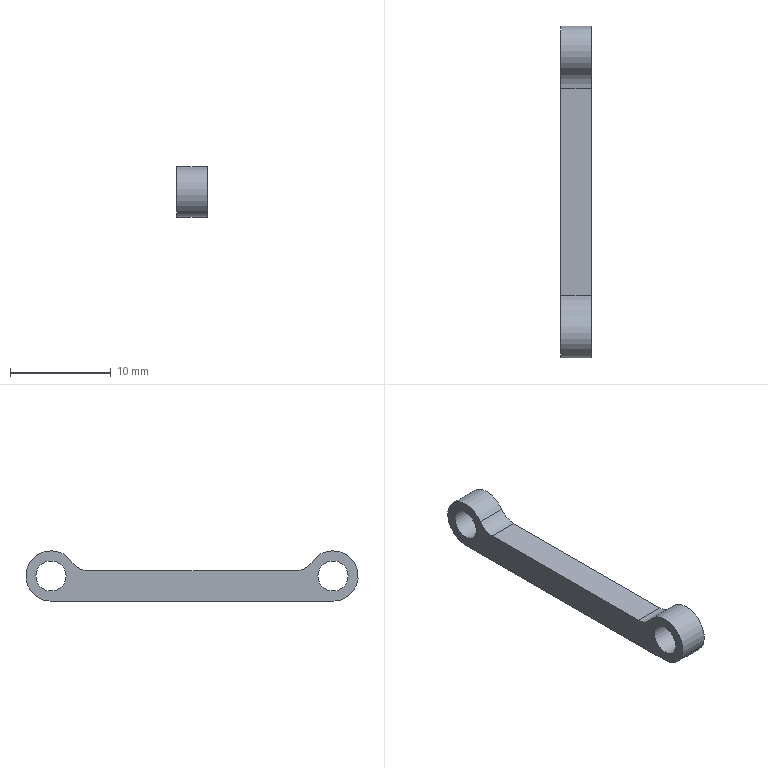Part | STEP file | 1-40.7 | 1 solid | 10 faces | box 3 x 33 x 5 mm | volume 291.958 mm3 | cylinder 6 | plane 4 | commonest cylinder face diameters 3 x2 4 x2 5 x2
STEP:
#1=CARTESIAN_POINT('',(0.,0.,0.));
#2=DIRECTION('',(0.,0.,1.));
#3=DIRECTION('',(1.,0.,0.));
#4=AXIS2_PLACEMENT_3D('',#1,#2,#3);
#5=CARTESIAN_POINT('',(0.,-14.,-2.5));
#6=VERTEX_POINT('',#5);
#7=CARTESIAN_POINT('',(0.,14.,-2.5));
#8=VERTEX_POINT('',#7);
#9=CARTESIAN_POINT('',(0.,-14.,-2.5));
#10=DIRECTION('',(0.,1.,0.));
#11=VECTOR('',#10,1.);
#12=LINE('',#9,#11);
#13=CARTESIAN_POINT('',(1.5,0.,-2.5));
#14=DIRECTION('',(0.,0.,-1.));
#15=DIRECTION('',(0.,1.,0.));
#16=AXIS2_PLACEMENT_3D('',#13,#14,#15);
#17=PLANE('',#16);
#18=CARTESIAN_POINT('',(-14.,-1.5));
#19=DIRECTION('',(1.,0.));
#20=VECTOR('',#19,1.);
#21=LINE('',#18,#20);
#22=(GEOMETRIC_REPRESENTATION_CONTEXT(2)PARAMETRIC_REPRESENTATION_CONTEXT()REPRESENTATION_CONTEXT('',''));
#23=DEFINITIONAL_REPRESENTATION('',(#21),#22);
#24=PCURVE('',#17,#23);
#25=CARTESIAN_POINT('',(0.,0.,14.151));
#26=DIRECTION('',(1.,0.,0.));
#27=DIRECTION('',(0.,1.,0.));
#28=AXIS2_PLACEMENT_3D('',#25,#26,#27);
#29=PLANE('',#28);
#30=CARTESIAN_POINT('',(-14.,-16.651));
#31=DIRECTION('',(1.,0.));
#32=VECTOR('',#31,1.);
#33=LINE('',#30,#32);
#34=(GEOMETRIC_REPRESENTATION_CONTEXT(2)PARAMETRIC_REPRESENTATION_CONTEXT()REPRESENTATION_CONTEXT('',''));
#35=DEFINITIONAL_REPRESENTATION('',(#33),#34);
#36=PCURVE('',#29,#35);
#37=SURFACE_CURVE('',#12,(#24,#36),.PCURVE_S1.);
#38=EDGE_CURVE('',#6,#8,#37,.T.);
#39=ORIENTED_EDGE('',*,*,#38,.T.);
#40=CARTESIAN_POINT('',(3.,14.,-2.5));
#41=VERTEX_POINT('',#40);
#42=CARTESIAN_POINT('',(0.,14.,-2.5));
#43=DIRECTION('',(1.,0.,0.));
#44=VECTOR('',#43,1.);
#45=LINE('',#42,#44);
#46=CARTESIAN_POINT('',(14.,-1.5));
#47=DIRECTION('',(0.,1.));
#48=VECTOR('',#47,1.);
#49=LINE('',#46,#48);
#50=(GEOMETRIC_REPRESENTATION_CONTEXT(2)PARAMETRIC_REPRESENTATION_CONTEXT()REPRESENTATION_CONTEXT('',''));
#51=DEFINITIONAL_REPRESENTATION('',(#49),#50);
#52=PCURVE('',#17,#51);
#53=CARTESIAN_POINT('',(0.,14.,0.));
#54=DIRECTION('',(1.,0.,0.));
#55=DIRECTION('',(0.,0.,-1.));
#56=AXIS2_PLACEMENT_3D('',#53,#54,#55);
#57=CYLINDRICAL_SURFACE('',#56,2.5);
#58=CARTESIAN_POINT('',(0.,0.));
#59=DIRECTION('',(0.,1.));
#60=VECTOR('',#59,1.);
#61=LINE('',#58,#60);
#62=(GEOMETRIC_REPRESENTATION_CONTEXT(2)PARAMETRIC_REPRESENTATION_CONTEXT()REPRESENTATION_CONTEXT('',''));
#63=DEFINITIONAL_REPRESENTATION('',(#61),#62);
#64=PCURVE('',#57,#63);
#65=SURFACE_CURVE('',#45,(#52,#64),.PCURVE_S1.);
#66=EDGE_CURVE('',#8,#41,#65,.T.);
#67=ORIENTED_EDGE('',*,*,#66,.T.);
#68=CARTESIAN_POINT('',(3.,-14.,-2.5));
#69=VERTEX_POINT('',#68);
#70=CARTESIAN_POINT('',(3.,-14.,-2.5));
#71=DIRECTION('',(0.,1.,0.));
#72=VECTOR('',#71,1.);
#73=LINE('',#70,#72);
#74=CARTESIAN_POINT('',(-14.,1.5));
#75=DIRECTION('',(1.,0.));
#76=VECTOR('',#75,1.);
#77=LINE('',#74,#76);
#78=(GEOMETRIC_REPRESENTATION_CONTEXT(2)PARAMETRIC_REPRESENTATION_CONTEXT()REPRESENTATION_CONTEXT('',''));
#79=DEFINITIONAL_REPRESENTATION('',(#77),#78);
#80=PCURVE('',#17,#79);
#81=CARTESIAN_POINT('',(3.,0.,14.151));
#82=DIRECTION('',(1.,0.,0.));
#83=DIRECTION('',(0.,1.,0.));
#84=AXIS2_PLACEMENT_3D('',#81,#82,#83);
#85=PLANE('',#84);
#86=CARTESIAN_POINT('',(-14.,-16.651));
#87=DIRECTION('',(1.,0.));
#88=VECTOR('',#87,1.);
#89=LINE('',#86,#88);
#90=(GEOMETRIC_REPRESENTATION_CONTEXT(2)PARAMETRIC_REPRESENTATION_CONTEXT()REPRESENTATION_CONTEXT('',''));
#91=DEFINITIONAL_REPRESENTATION('',(#89),#90);
#92=PCURVE('',#85,#91);
#93=SURFACE_CURVE('',#73,(#80,#92),.PCURVE_S1.);
#94=EDGE_CURVE('',#69,#41,#93,.T.);
#95=ORIENTED_EDGE('',*,*,#94,.F.);
#96=CARTESIAN_POINT('',(0.,-14.,-2.5));
#97=DIRECTION('',(1.,0.,0.));
#98=VECTOR('',#97,1.);
#99=LINE('',#96,#98);
#100=CARTESIAN_POINT('',(-14.,-1.5));
#101=DIRECTION('',(0.,1.));
#102=VECTOR('',#101,1.);
#103=LINE('',#100,#102);
#104=(GEOMETRIC_REPRESENTATION_CONTEXT(2)PARAMETRIC_REPRESENTATION_CONTEXT()REPRESENTATION_CONTEXT('',''));
#105=DEFINITIONAL_REPRESENTATION('',(#103),#104);
#106=PCURVE('',#17,#105);
#107=CARTESIAN_POINT('',(0.,-14.,0.));
#108=DIRECTION('',(1.,0.,0.));
#109=DIRECTION('',(0.,0.9798,0.2));
#110=AXIS2_PLACEMENT_3D('',#107,#108,#109);
#111=CYLINDRICAL_SURFACE('',#110,2.5);
#112=CARTESIAN_POINT('',(4.511,0.));
#113=DIRECTION('',(0.,1.));
#114=VECTOR('',#113,1.);
#115=LINE('',#112,#114);
#116=(GEOMETRIC_REPRESENTATION_CONTEXT(2)PARAMETRIC_REPRESENTATION_CONTEXT()REPRESENTATION_CONTEXT('',''));
#117=DEFINITIONAL_REPRESENTATION('',(#115),#116);
#118=PCURVE('',#111,#117);
#119=SURFACE_CURVE('',#99,(#106,#118),.PCURVE_S1.);
#120=EDGE_CURVE('',#6,#69,#119,.T.);
#121=ORIENTED_EDGE('',*,*,#120,.F.);
#122=EDGE_LOOP('',(#39,#67,#95,#121));
#123=FACE_BOUND('',#122,.T.);
#124=ADVANCED_FACE('',(#123),#17,.T.);
#125=CARTESIAN_POINT('',(0.,-12.5,0.));
#126=VERTEX_POINT('',#125);
#127=CARTESIAN_POINT('',(3.,-12.5,0.));
#128=VERTEX_POINT('',#127);
#129=CARTESIAN_POINT('',(0.,-12.5,0.));
#130=DIRECTION('',(1.,0.,0.));
#131=VECTOR('',#130,1.);
#132=LINE('',#129,#131);
#133=CARTESIAN_POINT('',(0.,-14.,0.));
#134=DIRECTION('',(1.,0.,0.));
#135=DIRECTION('',(0.,1.,0.));
#136=AXIS2_PLACEMENT_3D('',#133,#134,#135);
#137=CYLINDRICAL_SURFACE('',#136,1.5);
#138=CARTESIAN_POINT('',(6.283,0.));
#139=DIRECTION('',(0.,1.));
#140=VECTOR('',#139,1.);
#141=LINE('',#138,#140);
#142=(GEOMETRIC_REPRESENTATION_CONTEXT(2)PARAMETRIC_REPRESENTATION_CONTEXT()REPRESENTATION_CONTEXT('',''));
#143=DEFINITIONAL_REPRESENTATION('',(#141),#142);
#144=PCURVE('',#137,#143);
#145=CARTESIAN_POINT('',(0.,0.));
#146=DIRECTION('',(0.,1.));
#147=VECTOR('',#146,1.);
#148=LINE('',#145,#147);
#149=(GEOMETRIC_REPRESENTATION_CONTEXT(2)PARAMETRIC_REPRESENTATION_CONTEXT()REPRESENTATION_CONTEXT('',''));
#150=DEFINITIONAL_REPRESENTATION('',(#148),#149);
#151=PCURVE('',#137,#150);
#152=SEAM_CURVE('',#132,(#144,#151),.PCURVE_S1.);
#153=EDGE_CURVE('',#126,#128,#152,.T.);
#154=ORIENTED_EDGE('',*,*,#153,.T.);
#155=CARTESIAN_POINT('',(3.,-14.,0.));
#156=DIRECTION('',(-1.,0.,0.));
#157=DIRECTION('',(0.,1.,0.));
#158=AXIS2_PLACEMENT_3D('',#155,#156,#157);
#159=CIRCLE('',#158,1.5);
#160=CARTESIAN_POINT('',(6.283,3.));
#161=DIRECTION('',(-1.,0.));
#162=VECTOR('',#161,1.);
#163=LINE('',#160,#162);
#164=(GEOMETRIC_REPRESENTATION_CONTEXT(2)PARAMETRIC_REPRESENTATION_CONTEXT()REPRESENTATION_CONTEXT('',''));
#165=DEFINITIONAL_REPRESENTATION('',(#163),#164);
#166=PCURVE('',#137,#165);
#167=CARTESIAN_POINT('',(-12.5,-14.151));
#168=CARTESIAN_POINT('',(-12.5,-16.749));
#169=CARTESIAN_POINT('',(-14.75,-15.45));
#170=CARTESIAN_POINT('',(-17.,-14.151));
#171=CARTESIAN_POINT('',(-14.75,-12.852));
#172=CARTESIAN_POINT('',(-12.5,-11.553));
#173=CARTESIAN_POINT('',(-12.5,-14.151));
#174=(BOUNDED_CURVE()B_SPLINE_CURVE(2,(#167,#168,#169,#170,#171,#172,#173),.UNSPECIFIED.,.T.,.F.)B_SPLINE_CURVE_WITH_KNOTS((1,2,2,2,2,1),(-2.094,0.,2.094,4.189,6.283,8.378),.UNSPECIFIED.)CURVE()GEOMETRIC_REPRESENTATION_ITEM()RATIONAL_B_SPLINE_CURVE((1.,0.5,1.,0.5,1.,0.5,1.))REPRESENTATION_ITEM(''));
#175=(GEOMETRIC_REPRESENTATION_CONTEXT(2)PARAMETRIC_REPRESENTATION_CONTEXT()REPRESENTATION_CONTEXT('',''));
#176=DEFINITIONAL_REPRESENTATION('',(#174),#175);
#177=PCURVE('',#85,#176);
#178=SURFACE_CURVE('',#159,(#166,#177),.PCURVE_S1.);
#179=EDGE_CURVE('',#128,#128,#178,.T.);
#180=ORIENTED_EDGE('',*,*,#179,.T.);
#181=ORIENTED_EDGE('',*,*,#153,.F.);
#182=CARTESIAN_POINT('',(0.,-14.,0.));
#183=DIRECTION('',(-1.,0.,0.));
#184=DIRECTION('',(0.,1.,0.));
#185=AXIS2_PLACEMENT_3D('',#182,#183,#184);
#186=CIRCLE('',#185,1.5);
#187=CARTESIAN_POINT('',(6.283,0.));
#188=DIRECTION('',(-1.,0.));
#189=VECTOR('',#188,1.);
#190=LINE('',#187,#189);
#191=(GEOMETRIC_REPRESENTATION_CONTEXT(2)PARAMETRIC_REPRESENTATION_CONTEXT()REPRESENTATION_CONTEXT('',''));
#192=DEFINITIONAL_REPRESENTATION('',(#190),#191);
#193=PCURVE('',#137,#192);
#194=CARTESIAN_POINT('',(-12.5,-14.151));
#195=CARTESIAN_POINT('',(-12.5,-16.749));
#196=CARTESIAN_POINT('',(-14.75,-15.45));
#197=CARTESIAN_POINT('',(-17.,-14.151));
#198=CARTESIAN_POINT('',(-14.75,-12.852));
#199=CARTESIAN_POINT('',(-12.5,-11.553));
#200=CARTESIAN_POINT('',(-12.5,-14.151));
#201=(BOUNDED_CURVE()B_SPLINE_CURVE(2,(#194,#195,#196,#197,#198,#199,#200),.UNSPECIFIED.,.T.,.F.)B_SPLINE_CURVE_WITH_KNOTS((1,2,2,2,2,1),(-2.094,0.,2.094,4.189,6.283,8.378),.UNSPECIFIED.)CURVE()GEOMETRIC_REPRESENTATION_ITEM()RATIONAL_B_SPLINE_CURVE((1.,0.5,1.,0.5,1.,0.5,1.))REPRESENTATION_ITEM(''));
#202=(GEOMETRIC_REPRESENTATION_CONTEXT(2)PARAMETRIC_REPRESENTATION_CONTEXT()REPRESENTATION_CONTEXT('',''));
#203=DEFINITIONAL_REPRESENTATION('',(#201),#202);
#204=PCURVE('',#29,#203);
#205=SURFACE_CURVE('',#186,(#193,#204),.PCURVE_S1.);
#206=EDGE_CURVE('',#126,#126,#205,.T.);
#207=ORIENTED_EDGE('',*,*,#206,.F.);
#208=EDGE_LOOP('',(#154,#180,#181,#207));
#209=FACE_BOUND('',#208,.F.);
#210=ADVANCED_FACE('',(#209),#137,.F.);
#211=CARTESIAN_POINT('',(0.,15.5,0.));
#212=VERTEX_POINT('',#211);
#213=CARTESIAN_POINT('',(3.,15.5,0.));
#214=VERTEX_POINT('',#213);
#215=CARTESIAN_POINT('',(0.,15.5,0.));
#216=DIRECTION('',(1.,0.,0.));
#217=VECTOR('',#216,1.);
#218=LINE('',#215,#217);
#219=CARTESIAN_POINT('',(0.,14.,0.));
#220=DIRECTION('',(1.,0.,0.));
#221=DIRECTION('',(0.,1.,0.));
#222=AXIS2_PLACEMENT_3D('',#219,#220,#221);
#223=CYLINDRICAL_SURFACE('',#222,1.5);
#224=CARTESIAN_POINT('',(6.283,0.));
#225=DIRECTION('',(0.,1.));
#226=VECTOR('',#225,1.);
#227=LINE('',#224,#226);
#228=(GEOMETRIC_REPRESENTATION_CONTEXT(2)PARAMETRIC_REPRESENTATION_CONTEXT()REPRESENTATION_CONTEXT('',''));
#229=DEFINITIONAL_REPRESENTATION('',(#227),#228);
#230=PCURVE('',#223,#229);
#231=CARTESIAN_POINT('',(0.,0.));
#232=DIRECTION('',(0.,1.));
#233=VECTOR('',#232,1.);
#234=LINE('',#231,#233);
#235=(GEOMETRIC_REPRESENTATION_CONTEXT(2)PARAMETRIC_REPRESENTATION_CONTEXT()REPRESENTATION_CONTEXT('',''));
#236=DEFINITIONAL_REPRESENTATION('',(#234),#235);
#237=PCURVE('',#223,#236);
#238=SEAM_CURVE('',#218,(#230,#237),.PCURVE_S1.);
#239=EDGE_CURVE('',#212,#214,#238,.T.);
#240=ORIENTED_EDGE('',*,*,#239,.T.);
#241=CARTESIAN_POINT('',(3.,14.,0.));
#242=DIRECTION('',(-1.,0.,0.));
#243=DIRECTION('',(0.,1.,0.));
#244=AXIS2_PLACEMENT_3D('',#241,#242,#243);
#245=CIRCLE('',#244,1.5);
#246=CARTESIAN_POINT('',(6.283,3.));
#247=DIRECTION('',(-1.,0.));
#248=VECTOR('',#247,1.);
#249=LINE('',#246,#248);
#250=(GEOMETRIC_REPRESENTATION_CONTEXT(2)PARAMETRIC_REPRESENTATION_CONTEXT()REPRESENTATION_CONTEXT('',''));
#251=DEFINITIONAL_REPRESENTATION('',(#249),#250);
#252=PCURVE('',#223,#251);
#253=CARTESIAN_POINT('',(15.5,-14.151));
#254=CARTESIAN_POINT('',(15.5,-16.749));
#255=CARTESIAN_POINT('',(13.25,-15.45));
#256=CARTESIAN_POINT('',(11.,-14.151));
#257=CARTESIAN_POINT('',(13.25,-12.852));
#258=CARTESIAN_POINT('',(15.5,-11.553));
#259=CARTESIAN_POINT('',(15.5,-14.151));
#260=(BOUNDED_CURVE()B_SPLINE_CURVE(2,(#253,#254,#255,#256,#257,#258,#259),.UNSPECIFIED.,.T.,.F.)B_SPLINE_CURVE_WITH_KNOTS((1,2,2,2,2,1),(-2.094,0.,2.094,4.189,6.283,8.378),.UNSPECIFIED.)CURVE()GEOMETRIC_REPRESENTATION_ITEM()RATIONAL_B_SPLINE_CURVE((1.,0.5,1.,0.5,1.,0.5,1.))REPRESENTATION_ITEM(''));
#261=(GEOMETRIC_REPRESENTATION_CONTEXT(2)PARAMETRIC_REPRESENTATION_CONTEXT()REPRESENTATION_CONTEXT('',''));
#262=DEFINITIONAL_REPRESENTATION('',(#260),#261);
#263=PCURVE('',#85,#262);
#264=SURFACE_CURVE('',#245,(#252,#263),.PCURVE_S1.);
#265=EDGE_CURVE('',#214,#214,#264,.T.);
#266=ORIENTED_EDGE('',*,*,#265,.T.);
#267=ORIENTED_EDGE('',*,*,#239,.F.);
#268=CARTESIAN_POINT('',(0.,14.,0.));
#269=DIRECTION('',(-1.,0.,0.));
#270=DIRECTION('',(0.,1.,0.));
#271=AXIS2_PLACEMENT_3D('',#268,#269,#270);
#272=CIRCLE('',#271,1.5);
#273=CARTESIAN_POINT('',(6.283,0.));
#274=DIRECTION('',(-1.,0.));
#275=VECTOR('',#274,1.);
#276=LINE('',#273,#275);
#277=(GEOMETRIC_REPRESENTATION_CONTEXT(2)PARAMETRIC_REPRESENTATION_CONTEXT()REPRESENTATION_CONTEXT('',''));
#278=DEFINITIONAL_REPRESENTATION('',(#276),#277);
#279=PCURVE('',#223,#278);
#280=CARTESIAN_POINT('',(15.5,-14.151));
#281=CARTESIAN_POINT('',(15.5,-16.749));
#282=CARTESIAN_POINT('',(13.25,-15.45));
#283=CARTESIAN_POINT('',(11.,-14.151));
#284=CARTESIAN_POINT('',(13.25,-12.852));
#285=CARTESIAN_POINT('',(15.5,-11.553));
#286=CARTESIAN_POINT('',(15.5,-14.151));
#287=(BOUNDED_CURVE()B_SPLINE_CURVE(2,(#280,#281,#282,#283,#284,#285,#286),.UNSPECIFIED.,.T.,.F.)B_SPLINE_CURVE_WITH_KNOTS((1,2,2,2,2,1),(-2.094,0.,2.094,4.189,6.283,8.378),.UNSPECIFIED.)CURVE()GEOMETRIC_REPRESENTATION_ITEM()RATIONAL_B_SPLINE_CURVE((1.,0.5,1.,0.5,1.,0.5,1.))REPRESENTATION_ITEM(''));
#288=(GEOMETRIC_REPRESENTATION_CONTEXT(2)PARAMETRIC_REPRESENTATION_CONTEXT()REPRESENTATION_CONTEXT('',''));
#289=DEFINITIONAL_REPRESENTATION('',(#287),#288);
#290=PCURVE('',#29,#289);
#291=SURFACE_CURVE('',#272,(#279,#290),.PCURVE_S1.);
#292=EDGE_CURVE('',#212,#212,#291,.T.);
#293=ORIENTED_EDGE('',*,*,#292,.F.);
#294=EDGE_LOOP('',(#240,#266,#267,#293));
#295=FACE_BOUND('',#294,.F.);
#296=ADVANCED_FACE('',(#295),#223,.F.);
#297=CARTESIAN_POINT('',(0.,10.258,0.5));
#298=VERTEX_POINT('',#297);
#299=CARTESIAN_POINT('',(0.,-10.258,0.5));
#300=VERTEX_POINT('',#299);
#301=CARTESIAN_POINT('',(0.,10.258,0.5));
#302=DIRECTION('',(0.,-1.,0.));
#303=VECTOR('',#302,1.);
#304=LINE('',#301,#303);
#305=CARTESIAN_POINT('',(10.258,-13.651));
#306=DIRECTION('',(-1.,0.));
#307=VECTOR('',#306,1.);
#308=LINE('',#305,#307);
#309=(GEOMETRIC_REPRESENTATION_CONTEXT(2)PARAMETRIC_REPRESENTATION_CONTEXT()REPRESENTATION_CONTEXT('',''));
#310=DEFINITIONAL_REPRESENTATION('',(#308),#309);
#311=PCURVE('',#29,#310);
#312=CARTESIAN_POINT('',(1.5,0.,0.5));
#313=DIRECTION('',(0.,0.,1.));
#314=DIRECTION('',(0.,-1.,0.));
#315=AXIS2_PLACEMENT_3D('',#312,#313,#314);
#316=PLANE('',#315);
#317=CARTESIAN_POINT('',(-10.258,-1.5));
#318=DIRECTION('',(1.,0.));
#319=VECTOR('',#318,1.);
#320=LINE('',#317,#319);
#321=(GEOMETRIC_REPRESENTATION_CONTEXT(2)PARAMETRIC_REPRESENTATION_CONTEXT()REPRESENTATION_CONTEXT('',''));
#322=DEFINITIONAL_REPRESENTATION('',(#320),#321);
#323=PCURVE('',#316,#322);
#324=SURFACE_CURVE('',#304,(#311,#323),.PCURVE_S1.);
#325=EDGE_CURVE('',#298,#300,#324,.T.);
#326=ORIENTED_EDGE('',*,*,#325,.T.);
#327=CARTESIAN_POINT('',(0.,-11.921,1.389));
#328=VERTEX_POINT('',#327);
#329=CARTESIAN_POINT('',(0.,-10.258,2.5));
#330=DIRECTION('',(-1.,0.,0.));
#331=DIRECTION('',(0.,0.,-1.));
#332=AXIS2_PLACEMENT_3D('',#329,#330,#331);
#333=CIRCLE('',#332,2.);
#334=CARTESIAN_POINT('',(-10.258,-13.651));
#335=CARTESIAN_POINT('',(-13.722,-13.651));
#336=CARTESIAN_POINT('',(-11.99,-10.651));
#337=CARTESIAN_POINT('',(-10.258,-7.651));
#338=CARTESIAN_POINT('',(-8.526,-10.651));
#339=CARTESIAN_POINT('',(-6.794,-13.651));
#340=CARTESIAN_POINT('',(-10.258,-13.651));
#341=(BOUNDED_CURVE()B_SPLINE_CURVE(2,(#334,#335,#336,#337,#338,#339,#340),.UNSPECIFIED.,.T.,.F.)B_SPLINE_CURVE_WITH_KNOTS((1,2,2,2,2,1),(-2.094,0.,2.094,4.189,6.283,8.378),.UNSPECIFIED.)CURVE()GEOMETRIC_REPRESENTATION_ITEM()RATIONAL_B_SPLINE_CURVE((1.,0.5,1.,0.5,1.,0.5,1.))REPRESENTATION_ITEM(''));
#342=(GEOMETRIC_REPRESENTATION_CONTEXT(2)PARAMETRIC_REPRESENTATION_CONTEXT()REPRESENTATION_CONTEXT('',''));
#343=DEFINITIONAL_REPRESENTATION('',(#341),#342);
#344=PCURVE('',#29,#343);
#345=CARTESIAN_POINT('',(0.,-10.258,2.5));
#346=DIRECTION('',(1.,0.,0.));
#347=DIRECTION('',(0.,0.,-1.));
#348=AXIS2_PLACEMENT_3D('',#345,#346,#347);
#349=CYLINDRICAL_SURFACE('',#348,2.);
#350=CARTESIAN_POINT('',(6.283,0.));
#351=DIRECTION('',(-1.,0.));
#352=VECTOR('',#351,1.);
#353=LINE('',#350,#352);
#354=(GEOMETRIC_REPRESENTATION_CONTEXT(2)PARAMETRIC_REPRESENTATION_CONTEXT()REPRESENTATION_CONTEXT('',''));
#355=DEFINITIONAL_REPRESENTATION('',(#353),#354);
#356=PCURVE('',#349,#355);
#357=SURFACE_CURVE('',#333,(#344,#356),.PCURVE_S1.);
#358=EDGE_CURVE('',#300,#328,#357,.T.);
#359=ORIENTED_EDGE('',*,*,#358,.T.);
#360=CARTESIAN_POINT('',(0.,-14.,0.));
#361=DIRECTION('',(1.,0.,0.));
#362=DIRECTION('',(0.,0.8315,0.5556));
#363=AXIS2_PLACEMENT_3D('',#360,#361,#362);
#364=CIRCLE('',#363,2.5);
#365=CARTESIAN_POINT('',(-14.,-14.151));
#366=DIRECTION('',(0.8315,0.5556));
#367=AXIS2_PLACEMENT_2D('',#365,#366);
#368=CIRCLE('',#367,2.5);
#369=(GEOMETRIC_REPRESENTATION_CONTEXT(2)PARAMETRIC_REPRESENTATION_CONTEXT()REPRESENTATION_CONTEXT('',''));
#370=DEFINITIONAL_REPRESENTATION('',(#368),#369);
#371=PCURVE('',#29,#370);
#372=CARTESIAN_POINT('',(0.3877,0.));
#373=DIRECTION('',(1.,0.));
#374=VECTOR('',#373,1.);
#375=LINE('',#372,#374);
#376=(GEOMETRIC_REPRESENTATION_CONTEXT(2)PARAMETRIC_REPRESENTATION_CONTEXT()REPRESENTATION_CONTEXT('',''));
#377=DEFINITIONAL_REPRESENTATION('',(#375),#376);
#378=PCURVE('',#111,#377);
#379=SURFACE_CURVE('',#364,(#371,#378),.PCURVE_S1.);
#380=EDGE_CURVE('',#328,#6,#379,.T.);
#381=ORIENTED_EDGE('',*,*,#380,.T.);
#382=ORIENTED_EDGE('',*,*,#38,.T.);
#383=CARTESIAN_POINT('',(0.,11.921,1.389));
#384=VERTEX_POINT('',#383);
#385=CARTESIAN_POINT('',(0.,14.,0.));
#386=DIRECTION('',(1.,0.,0.));
#387=DIRECTION('',(0.,0.,-1.));
#388=AXIS2_PLACEMENT_3D('',#385,#386,#387);
#389=CIRCLE('',#388,2.5);
#390=CARTESIAN_POINT('',(14.,-14.151));
#391=DIRECTION('',(0.,-1.));
#392=AXIS2_PLACEMENT_2D('',#390,#391);
#393=CIRCLE('',#392,2.5);
#394=(GEOMETRIC_REPRESENTATION_CONTEXT(2)PARAMETRIC_REPRESENTATION_CONTEXT()REPRESENTATION_CONTEXT('',''));
#395=DEFINITIONAL_REPRESENTATION('',(#393),#394);
#396=PCURVE('',#29,#395);
#397=CARTESIAN_POINT('',(0.,0.));
#398=DIRECTION('',(1.,0.));
#399=VECTOR('',#398,1.);
#400=LINE('',#397,#399);
#401=(GEOMETRIC_REPRESENTATION_CONTEXT(2)PARAMETRIC_REPRESENTATION_CONTEXT()REPRESENTATION_CONTEXT('',''));
#402=DEFINITIONAL_REPRESENTATION('',(#400),#401);
#403=PCURVE('',#57,#402);
#404=SURFACE_CURVE('',#389,(#396,#403),.PCURVE_S1.);
#405=EDGE_CURVE('',#8,#384,#404,.T.);
#406=ORIENTED_EDGE('',*,*,#405,.T.);
#407=CARTESIAN_POINT('',(0.,10.258,2.5));
#408=DIRECTION('',(-1.,0.,0.));
#409=DIRECTION('',(0.,0.8315,-0.5556));
#410=AXIS2_PLACEMENT_3D('',#407,#408,#409);
#411=CIRCLE('',#410,2.);
#412=CARTESIAN_POINT('',(11.921,-12.762));
#413=CARTESIAN_POINT('',(9.997,-15.643));
#414=CARTESIAN_POINT('',(8.465,-12.536));
#415=CARTESIAN_POINT('',(6.932,-9.429));
#416=CARTESIAN_POINT('',(10.389,-9.655));
#417=CARTESIAN_POINT('',(13.846,-9.882));
#418=CARTESIAN_POINT('',(11.921,-12.762));
#419=(BOUNDED_CURVE()B_SPLINE_CURVE(2,(#412,#413,#414,#415,#416,#417,#418),.UNSPECIFIED.,.T.,.F.)B_SPLINE_CURVE_WITH_KNOTS((1,2,2,2,2,1),(-2.094,0.,2.094,4.189,6.283,8.378),.UNSPECIFIED.)CURVE()GEOMETRIC_REPRESENTATION_ITEM()RATIONAL_B_SPLINE_CURVE((1.,0.5,1.,0.5,1.,0.5,1.))REPRESENTATION_ITEM(''));
#420=(GEOMETRIC_REPRESENTATION_CONTEXT(2)PARAMETRIC_REPRESENTATION_CONTEXT()REPRESENTATION_CONTEXT('',''));
#421=DEFINITIONAL_REPRESENTATION('',(#419),#420);
#422=PCURVE('',#29,#421);
#423=CARTESIAN_POINT('',(0.,10.258,2.5));
#424=DIRECTION('',(1.,0.,0.));
#425=DIRECTION('',(0.,0.8315,-0.5556));
#426=AXIS2_PLACEMENT_3D('',#423,#424,#425);
#427=CYLINDRICAL_SURFACE('',#426,2.);
#428=CARTESIAN_POINT('',(6.283,0.));
#429=DIRECTION('',(-1.,0.));
#430=VECTOR('',#429,1.);
#431=LINE('',#428,#430);
#432=(GEOMETRIC_REPRESENTATION_CONTEXT(2)PARAMETRIC_REPRESENTATION_CONTEXT()REPRESENTATION_CONTEXT('',''));
#433=DEFINITIONAL_REPRESENTATION('',(#431),#432);
#434=PCURVE('',#427,#433);
#435=SURFACE_CURVE('',#411,(#422,#434),.PCURVE_S1.);
#436=EDGE_CURVE('',#384,#298,#435,.T.);
#437=ORIENTED_EDGE('',*,*,#436,.T.);
#438=EDGE_LOOP('',(#326,#359,#381,#382,#406,#437));
#439=FACE_BOUND('',#438,.F.);
#440=ORIENTED_EDGE('',*,*,#292,.T.);
#441=EDGE_LOOP('',(#440));
#442=FACE_BOUND('',#441,.F.);
#443=ORIENTED_EDGE('',*,*,#206,.T.);
#444=EDGE_LOOP('',(#443));
#445=FACE_BOUND('',#444,.F.);
#446=ADVANCED_FACE('',(#439,#442,#445),#29,.F.);
#447=CARTESIAN_POINT('',(3.,10.258,0.5));
#448=VERTEX_POINT('',#447);
#449=CARTESIAN_POINT('',(3.,-10.258,0.5));
#450=VERTEX_POINT('',#449);
#451=CARTESIAN_POINT('',(3.,10.258,0.5));
#452=DIRECTION('',(0.,-1.,0.));
#453=VECTOR('',#452,1.);
#454=LINE('',#451,#453);
#455=CARTESIAN_POINT('',(10.258,-13.651));
#456=DIRECTION('',(-1.,0.));
#457=VECTOR('',#456,1.);
#458=LINE('',#455,#457);
#459=(GEOMETRIC_REPRESENTATION_CONTEXT(2)PARAMETRIC_REPRESENTATION_CONTEXT()REPRESENTATION_CONTEXT('',''));
#460=DEFINITIONAL_REPRESENTATION('',(#458),#459);
#461=PCURVE('',#85,#460);
#462=CARTESIAN_POINT('',(-10.258,1.5));
#463=DIRECTION('',(1.,0.));
#464=VECTOR('',#463,1.);
#465=LINE('',#462,#464);
#466=(GEOMETRIC_REPRESENTATION_CONTEXT(2)PARAMETRIC_REPRESENTATION_CONTEXT()REPRESENTATION_CONTEXT('',''));
#467=DEFINITIONAL_REPRESENTATION('',(#465),#466);
#468=PCURVE('',#316,#467);
#469=SURFACE_CURVE('',#454,(#461,#468),.PCURVE_S1.);
#470=EDGE_CURVE('',#448,#450,#469,.T.);
#471=ORIENTED_EDGE('',*,*,#470,.T.);
#472=CARTESIAN_POINT('',(3.,-11.921,1.389));
#473=VERTEX_POINT('',#472);
#474=CARTESIAN_POINT('',(3.,-10.258,2.5));
#475=DIRECTION('',(-1.,0.,0.));
#476=DIRECTION('',(0.,0.,-1.));
#477=AXIS2_PLACEMENT_3D('',#474,#475,#476);
#478=CIRCLE('',#477,2.);
#479=CARTESIAN_POINT('',(-10.258,-13.651));
#480=CARTESIAN_POINT('',(-13.722,-13.651));
#481=CARTESIAN_POINT('',(-11.99,-10.651));
#482=CARTESIAN_POINT('',(-10.258,-7.651));
#483=CARTESIAN_POINT('',(-8.526,-10.651));
#484=CARTESIAN_POINT('',(-6.794,-13.651));
#485=CARTESIAN_POINT('',(-10.258,-13.651));
#486=(BOUNDED_CURVE()B_SPLINE_CURVE(2,(#479,#480,#481,#482,#483,#484,#485),.UNSPECIFIED.,.T.,.F.)B_SPLINE_CURVE_WITH_KNOTS((1,2,2,2,2,1),(-2.094,0.,2.094,4.189,6.283,8.378),.UNSPECIFIED.)CURVE()GEOMETRIC_REPRESENTATION_ITEM()RATIONAL_B_SPLINE_CURVE((1.,0.5,1.,0.5,1.,0.5,1.))REPRESENTATION_ITEM(''));
#487=(GEOMETRIC_REPRESENTATION_CONTEXT(2)PARAMETRIC_REPRESENTATION_CONTEXT()REPRESENTATION_CONTEXT('',''));
#488=DEFINITIONAL_REPRESENTATION('',(#486),#487);
#489=PCURVE('',#85,#488);
#490=CARTESIAN_POINT('',(6.283,3.));
#491=DIRECTION('',(-1.,0.));
#492=VECTOR('',#491,1.);
#493=LINE('',#490,#492);
#494=(GEOMETRIC_REPRESENTATION_CONTEXT(2)PARAMETRIC_REPRESENTATION_CONTEXT()REPRESENTATION_CONTEXT('',''));
#495=DEFINITIONAL_REPRESENTATION('',(#493),#494);
#496=PCURVE('',#349,#495);
#497=SURFACE_CURVE('',#478,(#489,#496),.PCURVE_S1.);
#498=EDGE_CURVE('',#450,#473,#497,.T.);
#499=ORIENTED_EDGE('',*,*,#498,.T.);
#500=CARTESIAN_POINT('',(3.,-14.,0.));
#501=DIRECTION('',(1.,0.,0.));
#502=DIRECTION('',(0.,0.8315,0.5556));
#503=AXIS2_PLACEMENT_3D('',#500,#501,#502);
#504=CIRCLE('',#503,2.5);
#505=CARTESIAN_POINT('',(-14.,-14.151));
#506=DIRECTION('',(0.8315,0.5556));
#507=AXIS2_PLACEMENT_2D('',#505,#506);
#508=CIRCLE('',#507,2.5);
#509=(GEOMETRIC_REPRESENTATION_CONTEXT(2)PARAMETRIC_REPRESENTATION_CONTEXT()REPRESENTATION_CONTEXT('',''));
#510=DEFINITIONAL_REPRESENTATION('',(#508),#509);
#511=PCURVE('',#85,#510);
#512=CARTESIAN_POINT('',(0.3877,3.));
#513=DIRECTION('',(1.,0.));
#514=VECTOR('',#513,1.);
#515=LINE('',#512,#514);
#516=(GEOMETRIC_REPRESENTATION_CONTEXT(2)PARAMETRIC_REPRESENTATION_CONTEXT()REPRESENTATION_CONTEXT('',''));
#517=DEFINITIONAL_REPRESENTATION('',(#515),#516);
#518=PCURVE('',#111,#517);
#519=SURFACE_CURVE('',#504,(#511,#518),.PCURVE_S1.);
#520=EDGE_CURVE('',#473,#69,#519,.T.);
#521=ORIENTED_EDGE('',*,*,#520,.T.);
#522=ORIENTED_EDGE('',*,*,#94,.T.);
#523=CARTESIAN_POINT('',(3.,11.921,1.389));
#524=VERTEX_POINT('',#523);
#525=CARTESIAN_POINT('',(3.,14.,0.));
#526=DIRECTION('',(1.,0.,0.));
#527=DIRECTION('',(0.,0.,-1.));
#528=AXIS2_PLACEMENT_3D('',#525,#526,#527);
#529=CIRCLE('',#528,2.5);
#530=CARTESIAN_POINT('',(14.,-14.151));
#531=DIRECTION('',(0.,-1.));
#532=AXIS2_PLACEMENT_2D('',#530,#531);
#533=CIRCLE('',#532,2.5);
#534=(GEOMETRIC_REPRESENTATION_CONTEXT(2)PARAMETRIC_REPRESENTATION_CONTEXT()REPRESENTATION_CONTEXT('',''));
#535=DEFINITIONAL_REPRESENTATION('',(#533),#534);
#536=PCURVE('',#85,#535);
#537=CARTESIAN_POINT('',(0.,3.));
#538=DIRECTION('',(1.,0.));
#539=VECTOR('',#538,1.);
#540=LINE('',#537,#539);
#541=(GEOMETRIC_REPRESENTATION_CONTEXT(2)PARAMETRIC_REPRESENTATION_CONTEXT()REPRESENTATION_CONTEXT('',''));
#542=DEFINITIONAL_REPRESENTATION('',(#540),#541);
#543=PCURVE('',#57,#542);
#544=SURFACE_CURVE('',#529,(#536,#543),.PCURVE_S1.);
#545=EDGE_CURVE('',#41,#524,#544,.T.);
#546=ORIENTED_EDGE('',*,*,#545,.T.);
#547=CARTESIAN_POINT('',(3.,10.258,2.5));
#548=DIRECTION('',(-1.,0.,0.));
#549=DIRECTION('',(0.,0.8315,-0.5556));
#550=AXIS2_PLACEMENT_3D('',#547,#548,#549);
#551=CIRCLE('',#550,2.);
#552=CARTESIAN_POINT('',(11.921,-12.762));
#553=CARTESIAN_POINT('',(9.997,-15.643));
#554=CARTESIAN_POINT('',(8.465,-12.536));
#555=CARTESIAN_POINT('',(6.932,-9.429));
#556=CARTESIAN_POINT('',(10.389,-9.655));
#557=CARTESIAN_POINT('',(13.846,-9.882));
#558=CARTESIAN_POINT('',(11.921,-12.762));
#559=(BOUNDED_CURVE()B_SPLINE_CURVE(2,(#552,#553,#554,#555,#556,#557,#558),.UNSPECIFIED.,.T.,.F.)B_SPLINE_CURVE_WITH_KNOTS((1,2,2,2,2,1),(-2.094,0.,2.094,4.189,6.283,8.378),.UNSPECIFIED.)CURVE()GEOMETRIC_REPRESENTATION_ITEM()RATIONAL_B_SPLINE_CURVE((1.,0.5,1.,0.5,1.,0.5,1.))REPRESENTATION_ITEM(''));
#560=(GEOMETRIC_REPRESENTATION_CONTEXT(2)PARAMETRIC_REPRESENTATION_CONTEXT()REPRESENTATION_CONTEXT('',''));
#561=DEFINITIONAL_REPRESENTATION('',(#559),#560);
#562=PCURVE('',#85,#561);
#563=CARTESIAN_POINT('',(6.283,3.));
#564=DIRECTION('',(-1.,0.));
#565=VECTOR('',#564,1.);
#566=LINE('',#563,#565);
#567=(GEOMETRIC_REPRESENTATION_CONTEXT(2)PARAMETRIC_REPRESENTATION_CONTEXT()REPRESENTATION_CONTEXT('',''));
#568=DEFINITIONAL_REPRESENTATION('',(#566),#567);
#569=PCURVE('',#427,#568);
#570=SURFACE_CURVE('',#551,(#562,#569),.PCURVE_S1.);
#571=EDGE_CURVE('',#524,#448,#570,.T.);
#572=ORIENTED_EDGE('',*,*,#571,.T.);
#573=EDGE_LOOP('',(#471,#499,#521,#522,#546,#572));
#574=FACE_BOUND('',#573,.T.);
#575=ORIENTED_EDGE('',*,*,#265,.T.);
#576=EDGE_LOOP('',(#575));
#577=FACE_BOUND('',#576,.T.);
#578=ORIENTED_EDGE('',*,*,#179,.T.);
#579=EDGE_LOOP('',(#578));
#580=FACE_BOUND('',#579,.T.);
#581=ADVANCED_FACE('',(#574,#577,#580),#85,.T.);
#582=ORIENTED_EDGE('',*,*,#520,.F.);
#583=CARTESIAN_POINT('',(0.,-11.921,1.389));
#584=DIRECTION('',(1.,0.,0.));
#585=VECTOR('',#584,1.);
#586=LINE('',#583,#585);
#587=CARTESIAN_POINT('',(0.3877,0.));
#588=DIRECTION('',(0.,1.));
#589=VECTOR('',#588,1.);
#590=LINE('',#587,#589);
#591=(GEOMETRIC_REPRESENTATION_CONTEXT(2)PARAMETRIC_REPRESENTATION_CONTEXT()REPRESENTATION_CONTEXT('',''));
#592=DEFINITIONAL_REPRESENTATION('',(#590),#591);
#593=PCURVE('',#111,#592);
#594=CARTESIAN_POINT('',(5.301,0.));
#595=DIRECTION('',(0.,1.));
#596=VECTOR('',#595,1.);
#597=LINE('',#594,#596);
#598=(GEOMETRIC_REPRESENTATION_CONTEXT(2)PARAMETRIC_REPRESENTATION_CONTEXT()REPRESENTATION_CONTEXT('',''));
#599=DEFINITIONAL_REPRESENTATION('',(#597),#598);
#600=PCURVE('',#349,#599);
#601=SURFACE_CURVE('',#586,(#593,#600),.PCURVE_S1.);
#602=EDGE_CURVE('',#328,#473,#601,.T.);
#603=ORIENTED_EDGE('',*,*,#602,.F.);
#604=ORIENTED_EDGE('',*,*,#380,.T.);
#605=ORIENTED_EDGE('',*,*,#120,.T.);
#606=EDGE_LOOP('',(#582,#603,#604,#605));
#607=FACE_BOUND('',#606,.T.);
#608=ADVANCED_FACE('',(#607),#111,.T.);
#609=ORIENTED_EDGE('',*,*,#405,.T.);
#610=CARTESIAN_POINT('',(0.,11.921,1.389));
#611=DIRECTION('',(1.,0.,0.));
#612=VECTOR('',#611,1.);
#613=LINE('',#610,#612);
#614=CARTESIAN_POINT('',(4.123,0.));
#615=DIRECTION('',(0.,1.));
#616=VECTOR('',#615,1.);
#617=LINE('',#614,#616);
#618=(GEOMETRIC_REPRESENTATION_CONTEXT(2)PARAMETRIC_REPRESENTATION_CONTEXT()REPRESENTATION_CONTEXT('',''));
#619=DEFINITIONAL_REPRESENTATION('',(#617),#618);
#620=PCURVE('',#57,#619);
#621=CARTESIAN_POINT('',(6.283,0.));
#622=DIRECTION('',(0.,1.));
#623=VECTOR('',#622,1.);
#624=LINE('',#621,#623);
#625=(GEOMETRIC_REPRESENTATION_CONTEXT(2)PARAMETRIC_REPRESENTATION_CONTEXT()REPRESENTATION_CONTEXT('',''));
#626=DEFINITIONAL_REPRESENTATION('',(#624),#625);
#627=PCURVE('',#427,#626);
#628=SURFACE_CURVE('',#613,(#620,#627),.PCURVE_S1.);
#629=EDGE_CURVE('',#384,#524,#628,.T.);
#630=ORIENTED_EDGE('',*,*,#629,.T.);
#631=ORIENTED_EDGE('',*,*,#545,.F.);
#632=ORIENTED_EDGE('',*,*,#66,.F.);
#633=EDGE_LOOP('',(#609,#630,#631,#632));
#634=FACE_BOUND('',#633,.T.);
#635=ADVANCED_FACE('',(#634),#57,.T.);
#636=ORIENTED_EDGE('',*,*,#325,.T.);
#637=CARTESIAN_POINT('',(0.,-10.258,0.5));
#638=DIRECTION('',(1.,0.,0.));
#639=VECTOR('',#638,1.);
#640=LINE('',#637,#639);
#641=CARTESIAN_POINT('',(10.258,-1.5));
#642=DIRECTION('',(0.,1.));
#643=VECTOR('',#642,1.);
#644=LINE('',#641,#643);
#645=(GEOMETRIC_REPRESENTATION_CONTEXT(2)PARAMETRIC_REPRESENTATION_CONTEXT()REPRESENTATION_CONTEXT('',''));
#646=DEFINITIONAL_REPRESENTATION('',(#644),#645);
#647=PCURVE('',#316,#646);
#648=CARTESIAN_POINT('',(6.283,0.));
#649=DIRECTION('',(0.,1.));
#650=VECTOR('',#649,1.);
#651=LINE('',#648,#650);
#652=(GEOMETRIC_REPRESENTATION_CONTEXT(2)PARAMETRIC_REPRESENTATION_CONTEXT()REPRESENTATION_CONTEXT('',''));
#653=DEFINITIONAL_REPRESENTATION('',(#651),#652);
#654=PCURVE('',#349,#653);
#655=SURFACE_CURVE('',#640,(#647,#654),.PCURVE_S1.);
#656=EDGE_CURVE('',#300,#450,#655,.T.);
#657=ORIENTED_EDGE('',*,*,#656,.T.);
#658=ORIENTED_EDGE('',*,*,#470,.F.);
#659=CARTESIAN_POINT('',(0.,10.258,0.5));
#660=DIRECTION('',(1.,0.,0.));
#661=VECTOR('',#660,1.);
#662=LINE('',#659,#661);
#663=CARTESIAN_POINT('',(-10.258,-1.5));
#664=DIRECTION('',(0.,1.));
#665=VECTOR('',#664,1.);
#666=LINE('',#663,#665);
#667=(GEOMETRIC_REPRESENTATION_CONTEXT(2)PARAMETRIC_REPRESENTATION_CONTEXT()REPRESENTATION_CONTEXT('',''));
#668=DEFINITIONAL_REPRESENTATION('',(#666),#667);
#669=PCURVE('',#316,#668);
#670=CARTESIAN_POINT('',(5.301,0.));
#671=DIRECTION('',(0.,1.));
#672=VECTOR('',#671,1.);
#673=LINE('',#670,#672);
#674=(GEOMETRIC_REPRESENTATION_CONTEXT(2)PARAMETRIC_REPRESENTATION_CONTEXT()REPRESENTATION_CONTEXT('',''));
#675=DEFINITIONAL_REPRESENTATION('',(#673),#674);
#676=PCURVE('',#427,#675);
#677=SURFACE_CURVE('',#662,(#669,#676),.PCURVE_S1.);
#678=EDGE_CURVE('',#298,#448,#677,.T.);
#679=ORIENTED_EDGE('',*,*,#678,.F.);
#680=EDGE_LOOP('',(#636,#657,#658,#679));
#681=FACE_BOUND('',#680,.T.);
#682=ADVANCED_FACE('',(#681),#316,.T.);
#683=ORIENTED_EDGE('',*,*,#656,.T.);
#684=ORIENTED_EDGE('',*,*,#498,.T.);
#685=ORIENTED_EDGE('',*,*,#602,.F.);
#686=ORIENTED_EDGE('',*,*,#358,.F.);
#687=EDGE_LOOP('',(#683,#684,#685,#686));
#688=FACE_BOUND('',#687,.F.);
#689=ADVANCED_FACE('',(#688),#349,.F.);
#690=ORIENTED_EDGE('',*,*,#629,.T.);
#691=ORIENTED_EDGE('',*,*,#571,.T.);
#692=ORIENTED_EDGE('',*,*,#678,.F.);
#693=ORIENTED_EDGE('',*,*,#436,.F.);
#694=EDGE_LOOP('',(#690,#691,#692,#693));
#695=FACE_BOUND('',#694,.F.);
#696=ADVANCED_FACE('',(#695),#427,.F.);
#697=CLOSED_SHELL('',(#124,#210,#296,#446,#581,#608,#635,#682,#689,#696));
#698=MANIFOLD_SOLID_BREP('',#697);
#699=(LENGTH_UNIT()NAMED_UNIT(*)SI_UNIT(.MILLI.,.METRE.));
#700=UNCERTAINTY_MEASURE_WITH_UNIT(LENGTH_MEASURE(0.0000001),#699,'','');
#701=(NAMED_UNIT(*)PLANE_ANGLE_UNIT()SI_UNIT($,.RADIAN.));
#702=(NAMED_UNIT(*)SI_UNIT($,.STERADIAN.)SOLID_ANGLE_UNIT());
#703=(GEOMETRIC_REPRESENTATION_CONTEXT(3)GLOBAL_UNCERTAINTY_ASSIGNED_CONTEXT((#700))GLOBAL_UNIT_ASSIGNED_CONTEXT((#699,#701,#702))REPRESENTATION_CONTEXT('',''));
#704=ADVANCED_BREP_SHAPE_REPRESENTATION('',(#4,#698),#703);